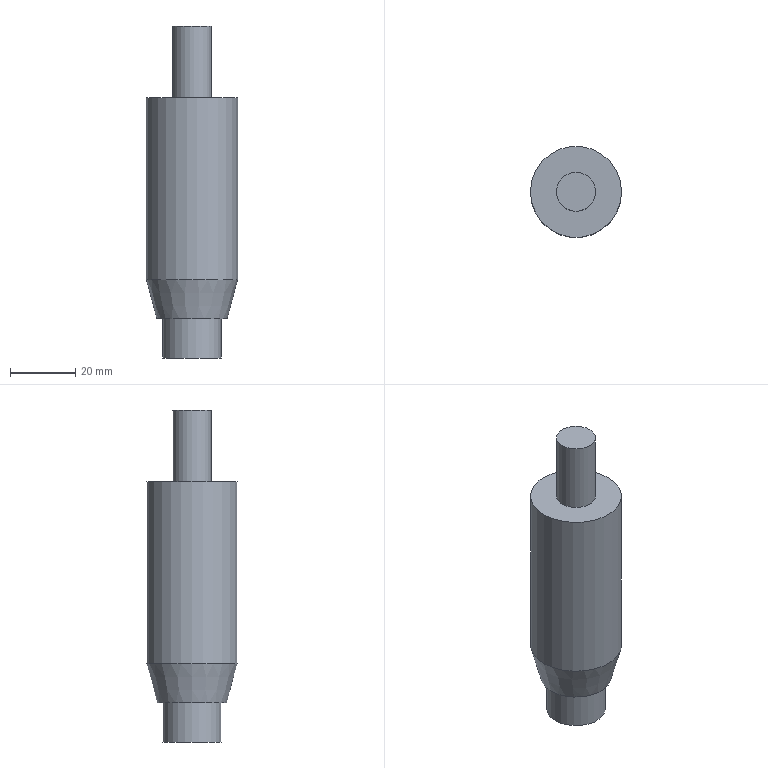Part | NX | features solid 2 | 1 solid | 8 faces | box 28 x 28 x 102 mm | volume 45846 mm3 | plane 4 | cylinder 3 | cone 1 | commonest cylinder face diameters 12 x1 18 x1 28 x1
STEP:
#1=CARTESIAN_POINT('',(591.,180.,332.));
#2=VERTEX_POINT('',#1);
#3=CARTESIAN_POINT('',(585.,180.,332.));
#4=DIRECTION('',(0.,0.,1.));
#5=DIRECTION('',(1.,0.,0.));
#6=AXIS2_PLACEMENT_3D('',#3,#4,#5);
#7=CIRCLE('',#6,6.);
#8=EDGE_CURVE('',#2,#2,#7,.T.);
#9=ORIENTED_EDGE('',*,*,#8,.T.);
#10=EDGE_LOOP('',(#9));
#11=FACE_BOUND('',#10,.T.);
#12=CARTESIAN_POINT('',(585.,184.75,332.));
#13=DIRECTION('',(0.,0.,-1.));
#14=DIRECTION('',(1.,0.,0.));
#15=AXIS2_PLACEMENT_3D('',#12,#13,#14);
#16=PLANE('',#15);
#17=ADVANCED_FACE('',(#11),#16,.F.);
#18=ORIENTED_EDGE('',*,*,#8,.F.);
#19=EDGE_LOOP('',(#18));
#20=FACE_BOUND('',#19,.T.);
#21=CARTESIAN_POINT('',(591.,180.,310.));
#22=VERTEX_POINT('',#21);
#23=CARTESIAN_POINT('',(585.,180.,310.));
#24=DIRECTION('',(0.,0.,1.));
#25=DIRECTION('',(1.,0.,0.));
#26=AXIS2_PLACEMENT_3D('',#23,#24,#25);
#27=CIRCLE('',#26,6.);
#28=EDGE_CURVE('',#22,#22,#27,.T.);
#29=ORIENTED_EDGE('',*,*,#28,.T.);
#30=EDGE_LOOP('',(#29));
#31=FACE_BOUND('',#30,.T.);
#32=CARTESIAN_POINT('',(585.,180.,332.));
#33=DIRECTION('',(0.,0.,-1.));
#34=DIRECTION('',(1.,0.,0.));
#35=AXIS2_PLACEMENT_3D('',#32,#33,#34);
#36=CYLINDRICAL_SURFACE('',#35,6.);
#37=ADVANCED_FACE('',(#20,#31),#36,.T.);
#38=CARTESIAN_POINT('',(599.,180.,310.));
#39=VERTEX_POINT('',#38);
#40=CARTESIAN_POINT('',(585.,180.,310.));
#41=DIRECTION('',(0.,0.,1.));
#42=DIRECTION('',(1.,0.,0.));
#43=AXIS2_PLACEMENT_3D('',#40,#41,#42);
#44=CIRCLE('',#43,14.);
#45=EDGE_CURVE('',#39,#39,#44,.T.);
#46=ORIENTED_EDGE('',*,*,#45,.T.);
#47=EDGE_LOOP('',(#46));
#48=FACE_BOUND('',#47,.T.);
#49=ORIENTED_EDGE('',*,*,#28,.F.);
#50=EDGE_LOOP('',(#49));
#51=FACE_BOUND('',#50,.T.);
#52=CARTESIAN_POINT('',(585.,186.,310.));
#53=DIRECTION('',(0.,0.,-1.));
#54=DIRECTION('',(1.,0.,0.));
#55=AXIS2_PLACEMENT_3D('',#52,#53,#54);
#56=PLANE('',#55);
#57=ADVANCED_FACE('',(#48,#51),#56,.F.);
#58=CARTESIAN_POINT('',(599.,180.,254.));
#59=VERTEX_POINT('',#58);
#60=CARTESIAN_POINT('',(585.,180.,254.));
#61=DIRECTION('',(0.,0.,1.));
#62=DIRECTION('',(1.,0.,0.));
#63=AXIS2_PLACEMENT_3D('',#60,#61,#62);
#64=CIRCLE('',#63,14.);
#65=EDGE_CURVE('',#59,#59,#64,.T.);
#66=ORIENTED_EDGE('',*,*,#65,.T.);
#67=EDGE_LOOP('',(#66));
#68=FACE_BOUND('',#67,.T.);
#69=ORIENTED_EDGE('',*,*,#45,.F.);
#70=EDGE_LOOP('',(#69));
#71=FACE_BOUND('',#70,.T.);
#72=CARTESIAN_POINT('',(585.,180.,332.));
#73=DIRECTION('',(0.,0.,-1.));
#74=DIRECTION('',(1.,0.,0.));
#75=AXIS2_PLACEMENT_3D('',#72,#73,#74);
#76=CYLINDRICAL_SURFACE('',#75,14.);
#77=ADVANCED_FACE('',(#68,#71),#76,.T.);
#78=CARTESIAN_POINT('',(595.785,180.,242.));
#79=VERTEX_POINT('',#78);
#80=CARTESIAN_POINT('',(585.,180.,242.));
#81=DIRECTION('',(0.,0.,1.));
#82=DIRECTION('',(1.,0.,0.));
#83=AXIS2_PLACEMENT_3D('',#80,#81,#82);
#84=CIRCLE('',#83,10.785);
#85=EDGE_CURVE('',#79,#79,#84,.T.);
#86=ORIENTED_EDGE('',*,*,#85,.T.);
#87=EDGE_LOOP('',(#86));
#88=FACE_BOUND('',#87,.T.);
#89=ORIENTED_EDGE('',*,*,#65,.F.);
#90=EDGE_LOOP('',(#89));
#91=FACE_BOUND('',#90,.T.);
#92=CARTESIAN_POINT('',(585.,180.,254.));
#93=DIRECTION('',(0.,0.,1.));
#94=DIRECTION('',(-1.,0.,0.));
#95=AXIS2_PLACEMENT_3D('',#92,#93,#94);
#96=CONICAL_SURFACE('',#95,14.,0.2618);
#97=ADVANCED_FACE('',(#88,#91),#96,.T.);
#98=ORIENTED_EDGE('',*,*,#85,.F.);
#99=EDGE_LOOP('',(#98));
#100=FACE_BOUND('',#99,.T.);
#101=CARTESIAN_POINT('',(594.,180.,242.));
#102=VERTEX_POINT('',#101);
#103=CARTESIAN_POINT('',(585.,180.,242.));
#104=DIRECTION('',(0.,0.,1.));
#105=DIRECTION('',(1.,0.,0.));
#106=AXIS2_PLACEMENT_3D('',#103,#104,#105);
#107=CIRCLE('',#106,9.);
#108=EDGE_CURVE('',#102,#102,#107,.T.);
#109=ORIENTED_EDGE('',*,*,#108,.T.);
#110=EDGE_LOOP('',(#109));
#111=FACE_BOUND('',#110,.T.);
#112=CARTESIAN_POINT('',(585.,189.,242.));
#113=DIRECTION('',(0.,0.,-1.));
#114=DIRECTION('',(1.,0.,0.));
#115=AXIS2_PLACEMENT_3D('',#112,#113,#114);
#116=PLANE('',#115);
#117=ADVANCED_FACE('',(#100,#111),#116,.T.);
#118=CARTESIAN_POINT('',(594.,180.,230.));
#119=VERTEX_POINT('',#118);
#120=CARTESIAN_POINT('',(585.,180.,230.));
#121=DIRECTION('',(0.,0.,1.));
#122=DIRECTION('',(1.,0.,0.));
#123=AXIS2_PLACEMENT_3D('',#120,#121,#122);
#124=CIRCLE('',#123,9.);
#125=EDGE_CURVE('',#119,#119,#124,.T.);
#126=ORIENTED_EDGE('',*,*,#125,.T.);
#127=EDGE_LOOP('',(#126));
#128=FACE_BOUND('',#127,.T.);
#129=ORIENTED_EDGE('',*,*,#108,.F.);
#130=EDGE_LOOP('',(#129));
#131=FACE_BOUND('',#130,.T.);
#132=CARTESIAN_POINT('',(585.,180.,332.));
#133=DIRECTION('',(0.,0.,-1.));
#134=DIRECTION('',(1.,0.,0.));
#135=AXIS2_PLACEMENT_3D('',#132,#133,#134);
#136=CYLINDRICAL_SURFACE('',#135,9.);
#137=ADVANCED_FACE('',(#128,#131),#136,.T.);
#138=ORIENTED_EDGE('',*,*,#125,.F.);
#139=EDGE_LOOP('',(#138));
#140=FACE_BOUND('',#139,.T.);
#141=CARTESIAN_POINT('',(585.,180.,230.));
#142=DIRECTION('',(0.,0.,-1.));
#143=DIRECTION('',(1.,0.,0.));
#144=AXIS2_PLACEMENT_3D('',#141,#142,#143);
#145=PLANE('',#144);
#146=ADVANCED_FACE('',(#140),#145,.T.);
#147=CLOSED_SHELL('',(#17,#37,#57,#77,#97,#117,#137,#146));
#148=MANIFOLD_SOLID_BREP('',#147);
#149=(LENGTH_UNIT()NAMED_UNIT(*)SI_UNIT(.MILLI.,.METRE.));
#150=UNCERTAINTY_MEASURE_WITH_UNIT(LENGTH_MEASURE(0.00001),#149,'','');
#151=(NAMED_UNIT(*)PLANE_ANGLE_UNIT()SI_UNIT($,.RADIAN.));
#152=(NAMED_UNIT(*)SI_UNIT($,.STERADIAN.)SOLID_ANGLE_UNIT());
#153=(GEOMETRIC_REPRESENTATION_CONTEXT(3)GLOBAL_UNCERTAINTY_ASSIGNED_CONTEXT((#150))GLOBAL_UNIT_ASSIGNED_CONTEXT((#149,#151,#152))REPRESENTATION_CONTEXT('',''));
#154=ADVANCED_BREP_SHAPE_REPRESENTATION('',(#148),#153);